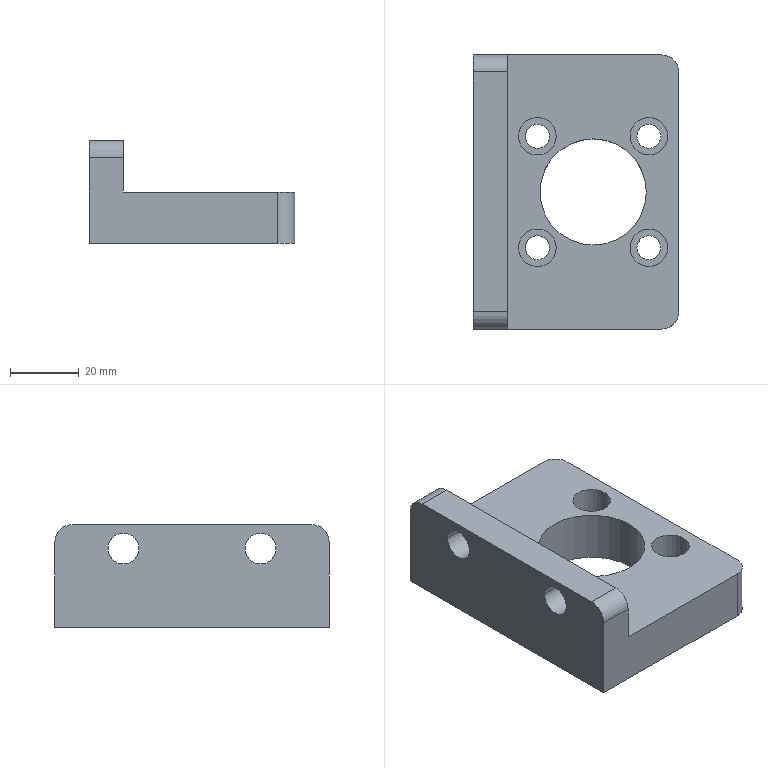Part | 1 solid | 38 faces | box 60 x 80 x 30 mm | volume 67019 mm3 | cylinder 26 | plane 12 | commonest cylinder face diameters 7 x8 11 x8 9 x4 10 x4 31 x2
STEP:
#1=CARTESIAN_POINT('',(-30.,-24.5,23.));
#2=VERTEX_POINT('',#1);
#3=CARTESIAN_POINT('',(-30.,-15.5,23.));
#4=VERTEX_POINT('',#3);
#5=CARTESIAN_POINT('',(-30.,-20.,23.));
#6=DIRECTION('',(1.,0.,0.));
#7=DIRECTION('',(0.,0.,-1.));
#8=AXIS2_PLACEMENT_3D('',#5,#6,#7);
#9=CIRCLE('',#8,4.5);
#10=EDGE_CURVE('',#2,#4,#9,.T.);
#11=ORIENTED_EDGE('',*,*,#10,.F.);
#12=CARTESIAN_POINT('',(-20.,-24.5,23.));
#13=VERTEX_POINT('',#12);
#14=CARTESIAN_POINT('',(-46.,-24.5,23.));
#15=DIRECTION('',(1.,0.,0.));
#16=VECTOR('',#15,1000.);
#17=LINE('',#14,#16);
#18=EDGE_CURVE('',#2,#13,#17,.T.);
#19=ORIENTED_EDGE('',*,*,#18,.T.);
#20=CARTESIAN_POINT('',(-20.,-15.5,23.));
#21=VERTEX_POINT('',#20);
#22=CARTESIAN_POINT('',(-20.,-20.,23.));
#23=DIRECTION('',(1.,0.,0.));
#24=DIRECTION('',(0.,1.,0.));
#25=AXIS2_PLACEMENT_3D('',#22,#23,#24);
#26=CIRCLE('',#25,4.5);
#27=EDGE_CURVE('',#13,#21,#26,.T.);
#28=ORIENTED_EDGE('',*,*,#27,.T.);
#29=CARTESIAN_POINT('',(-46.,-15.5,23.));
#30=DIRECTION('',(1.,0.,0.));
#31=VECTOR('',#30,1000.);
#32=LINE('',#29,#31);
#33=EDGE_CURVE('',#4,#21,#32,.T.);
#34=ORIENTED_EDGE('',*,*,#33,.F.);
#35=EDGE_LOOP('',(#11,#19,#28,#34));
#36=FACE_OUTER_BOUND('',#35,.T.);
#37=CARTESIAN_POINT('',(-46.,-20.,23.));
#38=DIRECTION('',(1.,0.,0.));
#39=DIRECTION('',(0.,1.,0.));
#40=AXIS2_PLACEMENT_3D('',#37,#38,#39);
#41=CYLINDRICAL_SURFACE('',#40,4.5);
#42=ADVANCED_FACE('',(#36),#41,.F.);
#43=CARTESIAN_POINT('',(-30.,15.5,23.));
#44=VERTEX_POINT('',#43);
#45=CARTESIAN_POINT('',(-30.,24.5,23.));
#46=VERTEX_POINT('',#45);
#47=CARTESIAN_POINT('',(-30.,20.,23.));
#48=DIRECTION('',(1.,0.,0.));
#49=DIRECTION('',(0.,0.,-1.));
#50=AXIS2_PLACEMENT_3D('',#47,#48,#49);
#51=CIRCLE('',#50,4.5);
#52=EDGE_CURVE('',#44,#46,#51,.T.);
#53=ORIENTED_EDGE('',*,*,#52,.F.);
#54=CARTESIAN_POINT('',(-20.,15.5,23.));
#55=VERTEX_POINT('',#54);
#56=CARTESIAN_POINT('',(-46.,15.5,23.));
#57=DIRECTION('',(1.,0.,0.));
#58=VECTOR('',#57,1000.);
#59=LINE('',#56,#58);
#60=EDGE_CURVE('',#44,#55,#59,.T.);
#61=ORIENTED_EDGE('',*,*,#60,.T.);
#62=CARTESIAN_POINT('',(-20.,24.5,23.));
#63=VERTEX_POINT('',#62);
#64=CARTESIAN_POINT('',(-20.,20.,23.));
#65=DIRECTION('',(1.,0.,0.));
#66=DIRECTION('',(0.,1.,0.));
#67=AXIS2_PLACEMENT_3D('',#64,#65,#66);
#68=CIRCLE('',#67,4.5);
#69=EDGE_CURVE('',#55,#63,#68,.T.);
#70=ORIENTED_EDGE('',*,*,#69,.T.);
#71=CARTESIAN_POINT('',(-46.,24.5,23.));
#72=DIRECTION('',(1.,0.,0.));
#73=VECTOR('',#72,1000.);
#74=LINE('',#71,#73);
#75=EDGE_CURVE('',#46,#63,#74,.T.);
#76=ORIENTED_EDGE('',*,*,#75,.F.);
#77=EDGE_LOOP('',(#53,#61,#70,#76));
#78=FACE_OUTER_BOUND('',#77,.T.);
#79=CARTESIAN_POINT('',(-46.,20.,23.));
#80=DIRECTION('',(1.,0.,0.));
#81=DIRECTION('',(0.,1.,0.));
#82=AXIS2_PLACEMENT_3D('',#79,#80,#81);
#83=CYLINDRICAL_SURFACE('',#82,4.5);
#84=ADVANCED_FACE('',(#78),#83,.F.);
#85=CARTESIAN_POINT('',(15.763,-16.263,7.));
#86=VERTEX_POINT('',#85);
#87=CARTESIAN_POINT('',(26.763,-16.263,7.));
#88=VERTEX_POINT('',#87);
#89=CARTESIAN_POINT('',(21.263,-16.263,7.));
#90=DIRECTION('',(0.,0.,1.));
#91=DIRECTION('',(1.,0.,0.));
#92=AXIS2_PLACEMENT_3D('',#89,#90,#91);
#93=CIRCLE('',#92,5.5);
#94=EDGE_CURVE('',#86,#88,#93,.T.);
#95=ORIENTED_EDGE('',*,*,#94,.F.);
#96=CARTESIAN_POINT('',(15.763,-16.263,15.));
#97=VERTEX_POINT('',#96);
#98=CARTESIAN_POINT('',(15.763,-16.263,7.));
#99=DIRECTION('',(0.,0.,1.));
#100=VECTOR('',#99,1000.);
#101=LINE('',#98,#100);
#102=EDGE_CURVE('',#86,#97,#101,.T.);
#103=ORIENTED_EDGE('',*,*,#102,.T.);
#104=CARTESIAN_POINT('',(26.763,-16.263,15.));
#105=VERTEX_POINT('',#104);
#106=CARTESIAN_POINT('',(21.263,-16.263,15.));
#107=DIRECTION('',(0.,0.,1.));
#108=DIRECTION('',(1.,0.,0.));
#109=AXIS2_PLACEMENT_3D('',#106,#107,#108);
#110=CIRCLE('',#109,5.5);
#111=EDGE_CURVE('',#97,#105,#110,.T.);
#112=ORIENTED_EDGE('',*,*,#111,.T.);
#113=CARTESIAN_POINT('',(26.763,-16.263,7.));
#114=DIRECTION('',(0.,0.,1.));
#115=VECTOR('',#114,1000.);
#116=LINE('',#113,#115);
#117=EDGE_CURVE('',#88,#105,#116,.T.);
#118=ORIENTED_EDGE('',*,*,#117,.F.);
#119=EDGE_LOOP('',(#95,#103,#112,#118));
#120=FACE_OUTER_BOUND('',#119,.T.);
#121=CARTESIAN_POINT('',(21.263,-16.263,7.));
#122=DIRECTION('',(0.,0.,1.));
#123=DIRECTION('',(1.,0.,0.));
#124=AXIS2_PLACEMENT_3D('',#121,#122,#123);
#125=CYLINDRICAL_SURFACE('',#124,5.5);
#126=ADVANCED_FACE('',(#120),#125,.F.);
#127=CARTESIAN_POINT('',(-16.763,-16.263,7.));
#128=VERTEX_POINT('',#127);
#129=CARTESIAN_POINT('',(-5.763,-16.263,7.));
#130=VERTEX_POINT('',#129);
#131=CARTESIAN_POINT('',(-11.263,-16.263,7.));
#132=DIRECTION('',(0.,0.,1.));
#133=DIRECTION('',(1.,0.,0.));
#134=AXIS2_PLACEMENT_3D('',#131,#132,#133);
#135=CIRCLE('',#134,5.5);
#136=EDGE_CURVE('',#128,#130,#135,.T.);
#137=ORIENTED_EDGE('',*,*,#136,.F.);
#138=CARTESIAN_POINT('',(-16.763,-16.263,15.));
#139=VERTEX_POINT('',#138);
#140=CARTESIAN_POINT('',(-16.763,-16.263,7.));
#141=DIRECTION('',(0.,0.,1.));
#142=VECTOR('',#141,1000.);
#143=LINE('',#140,#142);
#144=EDGE_CURVE('',#128,#139,#143,.T.);
#145=ORIENTED_EDGE('',*,*,#144,.T.);
#146=CARTESIAN_POINT('',(-5.763,-16.263,15.));
#147=VERTEX_POINT('',#146);
#148=CARTESIAN_POINT('',(-11.263,-16.263,15.));
#149=DIRECTION('',(0.,0.,1.));
#150=DIRECTION('',(1.,0.,0.));
#151=AXIS2_PLACEMENT_3D('',#148,#149,#150);
#152=CIRCLE('',#151,5.5);
#153=EDGE_CURVE('',#139,#147,#152,.T.);
#154=ORIENTED_EDGE('',*,*,#153,.T.);
#155=CARTESIAN_POINT('',(-5.763,-16.263,7.));
#156=DIRECTION('',(0.,0.,1.));
#157=VECTOR('',#156,1000.);
#158=LINE('',#155,#157);
#159=EDGE_CURVE('',#130,#147,#158,.T.);
#160=ORIENTED_EDGE('',*,*,#159,.F.);
#161=EDGE_LOOP('',(#137,#145,#154,#160));
#162=FACE_OUTER_BOUND('',#161,.T.);
#163=CARTESIAN_POINT('',(-11.263,-16.263,7.));
#164=DIRECTION('',(0.,0.,1.));
#165=DIRECTION('',(1.,0.,0.));
#166=AXIS2_PLACEMENT_3D('',#163,#164,#165);
#167=CYLINDRICAL_SURFACE('',#166,5.5);
#168=ADVANCED_FACE('',(#162),#167,.F.);
#169=CARTESIAN_POINT('',(15.763,16.263,7.));
#170=VERTEX_POINT('',#169);
#171=CARTESIAN_POINT('',(26.763,16.263,7.));
#172=VERTEX_POINT('',#171);
#173=CARTESIAN_POINT('',(21.263,16.263,7.));
#174=DIRECTION('',(0.,0.,1.));
#175=DIRECTION('',(1.,0.,0.));
#176=AXIS2_PLACEMENT_3D('',#173,#174,#175);
#177=CIRCLE('',#176,5.5);
#178=EDGE_CURVE('',#170,#172,#177,.T.);
#179=ORIENTED_EDGE('',*,*,#178,.F.);
#180=CARTESIAN_POINT('',(15.763,16.263,15.));
#181=VERTEX_POINT('',#180);
#182=CARTESIAN_POINT('',(15.763,16.263,7.));
#183=DIRECTION('',(0.,0.,1.));
#184=VECTOR('',#183,1000.);
#185=LINE('',#182,#184);
#186=EDGE_CURVE('',#170,#181,#185,.T.);
#187=ORIENTED_EDGE('',*,*,#186,.T.);
#188=CARTESIAN_POINT('',(26.763,16.263,15.));
#189=VERTEX_POINT('',#188);
#190=CARTESIAN_POINT('',(21.263,16.263,15.));
#191=DIRECTION('',(0.,0.,1.));
#192=DIRECTION('',(1.,0.,0.));
#193=AXIS2_PLACEMENT_3D('',#190,#191,#192);
#194=CIRCLE('',#193,5.5);
#195=EDGE_CURVE('',#181,#189,#194,.T.);
#196=ORIENTED_EDGE('',*,*,#195,.T.);
#197=CARTESIAN_POINT('',(26.763,16.263,7.));
#198=DIRECTION('',(0.,0.,1.));
#199=VECTOR('',#198,1000.);
#200=LINE('',#197,#199);
#201=EDGE_CURVE('',#172,#189,#200,.T.);
#202=ORIENTED_EDGE('',*,*,#201,.F.);
#203=EDGE_LOOP('',(#179,#187,#196,#202));
#204=FACE_OUTER_BOUND('',#203,.T.);
#205=CARTESIAN_POINT('',(21.263,16.263,7.));
#206=DIRECTION('',(0.,0.,1.));
#207=DIRECTION('',(1.,0.,0.));
#208=AXIS2_PLACEMENT_3D('',#205,#206,#207);
#209=CYLINDRICAL_SURFACE('',#208,5.5);
#210=ADVANCED_FACE('',(#204),#209,.F.);
#211=CARTESIAN_POINT('',(-16.763,16.263,7.));
#212=VERTEX_POINT('',#211);
#213=CARTESIAN_POINT('',(-5.763,16.263,7.));
#214=VERTEX_POINT('',#213);
#215=CARTESIAN_POINT('',(-11.263,16.263,7.));
#216=DIRECTION('',(0.,0.,1.));
#217=DIRECTION('',(1.,0.,0.));
#218=AXIS2_PLACEMENT_3D('',#215,#216,#217);
#219=CIRCLE('',#218,5.5);
#220=EDGE_CURVE('',#212,#214,#219,.T.);
#221=ORIENTED_EDGE('',*,*,#220,.F.);
#222=CARTESIAN_POINT('',(-16.763,16.263,15.));
#223=VERTEX_POINT('',#222);
#224=CARTESIAN_POINT('',(-16.763,16.263,7.));
#225=DIRECTION('',(0.,0.,1.));
#226=VECTOR('',#225,1000.);
#227=LINE('',#224,#226);
#228=EDGE_CURVE('',#212,#223,#227,.T.);
#229=ORIENTED_EDGE('',*,*,#228,.T.);
#230=CARTESIAN_POINT('',(-5.763,16.263,15.));
#231=VERTEX_POINT('',#230);
#232=CARTESIAN_POINT('',(-11.263,16.263,15.));
#233=DIRECTION('',(0.,0.,1.));
#234=DIRECTION('',(1.,0.,0.));
#235=AXIS2_PLACEMENT_3D('',#232,#233,#234);
#236=CIRCLE('',#235,5.5);
#237=EDGE_CURVE('',#223,#231,#236,.T.);
#238=ORIENTED_EDGE('',*,*,#237,.T.);
#239=CARTESIAN_POINT('',(-5.763,16.263,7.));
#240=DIRECTION('',(0.,0.,1.));
#241=VECTOR('',#240,1000.);
#242=LINE('',#239,#241);
#243=EDGE_CURVE('',#214,#231,#242,.T.);
#244=ORIENTED_EDGE('',*,*,#243,.F.);
#245=EDGE_LOOP('',(#221,#229,#238,#244));
#246=FACE_OUTER_BOUND('',#245,.T.);
#247=CARTESIAN_POINT('',(-11.263,16.263,7.));
#248=DIRECTION('',(0.,0.,1.));
#249=DIRECTION('',(1.,0.,0.));
#250=AXIS2_PLACEMENT_3D('',#247,#248,#249);
#251=CYLINDRICAL_SURFACE('',#250,5.5);
#252=ADVANCED_FACE('',(#246),#251,.F.);
#253=CARTESIAN_POINT('',(-10.5,0.,0.));
#254=VERTEX_POINT('',#253);
#255=CARTESIAN_POINT('',(20.5,0.,0.));
#256=VERTEX_POINT('',#255);
#257=CARTESIAN_POINT('',(5.,0.,0.));
#258=DIRECTION('',(0.,0.,1.));
#259=DIRECTION('',(1.,0.,0.));
#260=AXIS2_PLACEMENT_3D('',#257,#258,#259);
#261=CIRCLE('',#260,15.5);
#262=EDGE_CURVE('',#254,#256,#261,.T.);
#263=ORIENTED_EDGE('',*,*,#262,.F.);
#264=CARTESIAN_POINT('',(-10.5,0.,15.));
#265=VERTEX_POINT('',#264);
#266=CARTESIAN_POINT('',(-10.5,0.,0.));
#267=DIRECTION('',(0.,0.,1.));
#268=VECTOR('',#267,1000.);
#269=LINE('',#266,#268);
#270=EDGE_CURVE('',#254,#265,#269,.T.);
#271=ORIENTED_EDGE('',*,*,#270,.T.);
#272=CARTESIAN_POINT('',(20.5,0.,15.));
#273=VERTEX_POINT('',#272);
#274=CARTESIAN_POINT('',(5.,0.,15.));
#275=DIRECTION('',(0.,0.,1.));
#276=DIRECTION('',(1.,0.,0.));
#277=AXIS2_PLACEMENT_3D('',#274,#275,#276);
#278=CIRCLE('',#277,15.5);
#279=EDGE_CURVE('',#265,#273,#278,.T.);
#280=ORIENTED_EDGE('',*,*,#279,.T.);
#281=CARTESIAN_POINT('',(20.5,0.,0.));
#282=DIRECTION('',(0.,0.,1.));
#283=VECTOR('',#282,1000.);
#284=LINE('',#281,#283);
#285=EDGE_CURVE('',#256,#273,#284,.T.);
#286=ORIENTED_EDGE('',*,*,#285,.F.);
#287=EDGE_LOOP('',(#263,#271,#280,#286));
#288=FACE_OUTER_BOUND('',#287,.T.);
#289=CARTESIAN_POINT('',(5.,0.,0.));
#290=DIRECTION('',(0.,0.,1.));
#291=DIRECTION('',(1.,0.,0.));
#292=AXIS2_PLACEMENT_3D('',#289,#290,#291);
#293=CYLINDRICAL_SURFACE('',#292,15.5);
#294=ADVANCED_FACE('',(#288),#293,.F.);
#295=CARTESIAN_POINT('',(-14.763,16.263,0.));
#296=VERTEX_POINT('',#295);
#297=CARTESIAN_POINT('',(-7.763,16.263,0.));
#298=VERTEX_POINT('',#297);
#299=CARTESIAN_POINT('',(-11.263,16.263,0.));
#300=DIRECTION('',(0.,0.,1.));
#301=DIRECTION('',(-1.,0.,0.));
#302=AXIS2_PLACEMENT_3D('',#299,#300,#301);
#303=CIRCLE('',#302,3.5);
#304=EDGE_CURVE('',#296,#298,#303,.T.);
#305=ORIENTED_EDGE('',*,*,#304,.F.);
#306=CARTESIAN_POINT('',(-14.763,16.263,7.));
#307=VERTEX_POINT('',#306);
#308=CARTESIAN_POINT('',(-14.763,16.263,0.));
#309=DIRECTION('',(0.,0.,1.));
#310=VECTOR('',#309,1000.);
#311=LINE('',#308,#310);
#312=EDGE_CURVE('',#296,#307,#311,.T.);
#313=ORIENTED_EDGE('',*,*,#312,.T.);
#314=CARTESIAN_POINT('',(-7.763,16.263,7.));
#315=VERTEX_POINT('',#314);
#316=CARTESIAN_POINT('',(-11.263,16.263,7.));
#317=DIRECTION('',(0.,0.,-1.));
#318=DIRECTION('',(1.,0.,0.));
#319=AXIS2_PLACEMENT_3D('',#316,#317,#318);
#320=CIRCLE('',#319,3.5);
#321=EDGE_CURVE('',#315,#307,#320,.T.);
#322=ORIENTED_EDGE('',*,*,#321,.F.);
#323=CARTESIAN_POINT('',(-7.763,16.263,0.));
#324=DIRECTION('',(0.,0.,1.));
#325=VECTOR('',#324,1000.);
#326=LINE('',#323,#325);
#327=EDGE_CURVE('',#298,#315,#326,.T.);
#328=ORIENTED_EDGE('',*,*,#327,.F.);
#329=EDGE_LOOP('',(#305,#313,#322,#328));
#330=FACE_OUTER_BOUND('',#329,.T.);
#331=CARTESIAN_POINT('',(-11.263,16.263,0.));
#332=DIRECTION('',(0.,0.,1.));
#333=DIRECTION('',(1.,0.,0.));
#334=AXIS2_PLACEMENT_3D('',#331,#332,#333);
#335=CYLINDRICAL_SURFACE('',#334,3.5);
#336=ADVANCED_FACE('',(#330),#335,.F.);
#337=CARTESIAN_POINT('',(17.763,16.263,0.));
#338=VERTEX_POINT('',#337);
#339=CARTESIAN_POINT('',(24.763,16.263,0.));
#340=VERTEX_POINT('',#339);
#341=CARTESIAN_POINT('',(21.263,16.263,0.));
#342=DIRECTION('',(0.,0.,1.));
#343=DIRECTION('',(1.,0.,0.));
#344=AXIS2_PLACEMENT_3D('',#341,#342,#343);
#345=CIRCLE('',#344,3.5);
#346=EDGE_CURVE('',#338,#340,#345,.T.);
#347=ORIENTED_EDGE('',*,*,#346,.F.);
#348=CARTESIAN_POINT('',(17.763,16.263,7.));
#349=VERTEX_POINT('',#348);
#350=CARTESIAN_POINT('',(17.763,16.263,0.));
#351=DIRECTION('',(0.,0.,1.));
#352=VECTOR('',#351,1000.);
#353=LINE('',#350,#352);
#354=EDGE_CURVE('',#338,#349,#353,.T.);
#355=ORIENTED_EDGE('',*,*,#354,.T.);
#356=CARTESIAN_POINT('',(24.763,16.263,7.));
#357=VERTEX_POINT('',#356);
#358=CARTESIAN_POINT('',(21.263,16.263,7.));
#359=DIRECTION('',(0.,0.,-1.));
#360=DIRECTION('',(1.,0.,0.));
#361=AXIS2_PLACEMENT_3D('',#358,#359,#360);
#362=CIRCLE('',#361,3.5);
#363=EDGE_CURVE('',#357,#349,#362,.T.);
#364=ORIENTED_EDGE('',*,*,#363,.F.);
#365=CARTESIAN_POINT('',(24.763,16.263,0.));
#366=DIRECTION('',(0.,0.,1.));
#367=VECTOR('',#366,1000.);
#368=LINE('',#365,#367);
#369=EDGE_CURVE('',#340,#357,#368,.T.);
#370=ORIENTED_EDGE('',*,*,#369,.F.);
#371=EDGE_LOOP('',(#347,#355,#364,#370));
#372=FACE_OUTER_BOUND('',#371,.T.);
#373=CARTESIAN_POINT('',(21.263,16.263,0.));
#374=DIRECTION('',(0.,0.,1.));
#375=DIRECTION('',(1.,0.,0.));
#376=AXIS2_PLACEMENT_3D('',#373,#374,#375);
#377=CYLINDRICAL_SURFACE('',#376,3.5);
#378=ADVANCED_FACE('',(#372),#377,.F.);
#379=CARTESIAN_POINT('',(-14.763,-16.263,0.));
#380=VERTEX_POINT('',#379);
#381=CARTESIAN_POINT('',(-7.763,-16.263,0.));
#382=VERTEX_POINT('',#381);
#383=CARTESIAN_POINT('',(-11.263,-16.263,0.));
#384=DIRECTION('',(0.,0.,1.));
#385=DIRECTION('',(1.,0.,0.));
#386=AXIS2_PLACEMENT_3D('',#383,#384,#385);
#387=CIRCLE('',#386,3.5);
#388=EDGE_CURVE('',#380,#382,#387,.T.);
#389=ORIENTED_EDGE('',*,*,#388,.F.);
#390=CARTESIAN_POINT('',(-14.763,-16.263,7.));
#391=VERTEX_POINT('',#390);
#392=CARTESIAN_POINT('',(-14.763,-16.263,0.));
#393=DIRECTION('',(0.,0.,1.));
#394=VECTOR('',#393,1000.);
#395=LINE('',#392,#394);
#396=EDGE_CURVE('',#380,#391,#395,.T.);
#397=ORIENTED_EDGE('',*,*,#396,.T.);
#398=CARTESIAN_POINT('',(-7.763,-16.263,7.));
#399=VERTEX_POINT('',#398);
#400=CARTESIAN_POINT('',(-11.263,-16.263,7.));
#401=DIRECTION('',(0.,0.,-1.));
#402=DIRECTION('',(1.,0.,0.));
#403=AXIS2_PLACEMENT_3D('',#400,#401,#402);
#404=CIRCLE('',#403,3.5);
#405=EDGE_CURVE('',#399,#391,#404,.T.);
#406=ORIENTED_EDGE('',*,*,#405,.F.);
#407=CARTESIAN_POINT('',(-7.763,-16.263,0.));
#408=DIRECTION('',(0.,0.,1.));
#409=VECTOR('',#408,1000.);
#410=LINE('',#407,#409);
#411=EDGE_CURVE('',#382,#399,#410,.T.);
#412=ORIENTED_EDGE('',*,*,#411,.F.);
#413=EDGE_LOOP('',(#389,#397,#406,#412));
#414=FACE_OUTER_BOUND('',#413,.T.);
#415=CARTESIAN_POINT('',(-11.263,-16.263,0.));
#416=DIRECTION('',(0.,0.,1.));
#417=DIRECTION('',(1.,0.,0.));
#418=AXIS2_PLACEMENT_3D('',#415,#416,#417);
#419=CYLINDRICAL_SURFACE('',#418,3.5);
#420=ADVANCED_FACE('',(#414),#419,.F.);
#421=CARTESIAN_POINT('',(17.763,-16.263,0.));
#422=VERTEX_POINT('',#421);
#423=CARTESIAN_POINT('',(24.763,-16.263,0.));
#424=VERTEX_POINT('',#423);
#425=CARTESIAN_POINT('',(21.263,-16.263,0.));
#426=DIRECTION('',(0.,0.,1.));
#427=DIRECTION('',(-1.,0.,0.));
#428=AXIS2_PLACEMENT_3D('',#425,#426,#427);
#429=CIRCLE('',#428,3.5);
#430=EDGE_CURVE('',#422,#424,#429,.T.);
#431=ORIENTED_EDGE('',*,*,#430,.F.);
#432=CARTESIAN_POINT('',(17.763,-16.263,7.));
#433=VERTEX_POINT('',#432);
#434=CARTESIAN_POINT('',(17.763,-16.263,0.));
#435=DIRECTION('',(0.,0.,1.));
#436=VECTOR('',#435,1000.);
#437=LINE('',#434,#436);
#438=EDGE_CURVE('',#422,#433,#437,.T.);
#439=ORIENTED_EDGE('',*,*,#438,.T.);
#440=CARTESIAN_POINT('',(24.763,-16.263,7.));
#441=VERTEX_POINT('',#440);
#442=CARTESIAN_POINT('',(21.263,-16.263,7.));
#443=DIRECTION('',(0.,0.,-1.));
#444=DIRECTION('',(1.,0.,0.));
#445=AXIS2_PLACEMENT_3D('',#442,#443,#444);
#446=CIRCLE('',#445,3.5);
#447=EDGE_CURVE('',#441,#433,#446,.T.);
#448=ORIENTED_EDGE('',*,*,#447,.F.);
#449=CARTESIAN_POINT('',(24.763,-16.263,0.));
#450=DIRECTION('',(0.,0.,1.));
#451=VECTOR('',#450,1000.);
#452=LINE('',#449,#451);
#453=EDGE_CURVE('',#424,#441,#452,.T.);
#454=ORIENTED_EDGE('',*,*,#453,.F.);
#455=EDGE_LOOP('',(#431,#439,#448,#454));
#456=FACE_OUTER_BOUND('',#455,.T.);
#457=CARTESIAN_POINT('',(21.263,-16.263,0.));
#458=DIRECTION('',(0.,0.,1.));
#459=DIRECTION('',(1.,0.,0.));
#460=AXIS2_PLACEMENT_3D('',#457,#458,#459);
#461=CYLINDRICAL_SURFACE('',#460,3.5);
#462=ADVANCED_FACE('',(#456),#461,.F.);
#463=ORIENTED_EDGE('',*,*,#438,.F.);
#464=CARTESIAN_POINT('',(21.263,-16.263,0.));
#465=DIRECTION('',(0.,0.,1.));
#466=DIRECTION('',(-1.,0.,0.));
#467=AXIS2_PLACEMENT_3D('',#464,#465,#466);
#468=CIRCLE('',#467,3.5);
#469=EDGE_CURVE('',#424,#422,#468,.T.);
#470=ORIENTED_EDGE('',*,*,#469,.F.);
#471=ORIENTED_EDGE('',*,*,#453,.T.);
#472=CARTESIAN_POINT('',(21.263,-16.263,7.));
#473=DIRECTION('',(0.,0.,-1.));
#474=DIRECTION('',(1.,0.,0.));
#475=AXIS2_PLACEMENT_3D('',#472,#473,#474);
#476=CIRCLE('',#475,3.5);
#477=EDGE_CURVE('',#433,#441,#476,.T.);
#478=ORIENTED_EDGE('',*,*,#477,.F.);
#479=EDGE_LOOP('',(#463,#470,#471,#478));
#480=FACE_OUTER_BOUND('',#479,.T.);
#481=CARTESIAN_POINT('',(21.263,-16.263,0.));
#482=DIRECTION('',(0.,0.,1.));
#483=DIRECTION('',(1.,0.,0.));
#484=AXIS2_PLACEMENT_3D('',#481,#482,#483);
#485=CYLINDRICAL_SURFACE('',#484,3.5);
#486=ADVANCED_FACE('',(#480),#485,.F.);
#487=ORIENTED_EDGE('',*,*,#396,.F.);
#488=CARTESIAN_POINT('',(-11.263,-16.263,0.));
#489=DIRECTION('',(0.,0.,1.));
#490=DIRECTION('',(1.,0.,0.));
#491=AXIS2_PLACEMENT_3D('',#488,#489,#490);
#492=CIRCLE('',#491,3.5);
#493=EDGE_CURVE('',#382,#380,#492,.T.);
#494=ORIENTED_EDGE('',*,*,#493,.F.);
#495=ORIENTED_EDGE('',*,*,#411,.T.);
#496=CARTESIAN_POINT('',(-11.263,-16.263,7.));
#497=DIRECTION('',(0.,0.,-1.));
#498=DIRECTION('',(1.,0.,0.));
#499=AXIS2_PLACEMENT_3D('',#496,#497,#498);
#500=CIRCLE('',#499,3.5);
#501=EDGE_CURVE('',#391,#399,#500,.T.);
#502=ORIENTED_EDGE('',*,*,#501,.F.);
#503=EDGE_LOOP('',(#487,#494,#495,#502));
#504=FACE_OUTER_BOUND('',#503,.T.);
#505=CARTESIAN_POINT('',(-11.263,-16.263,0.));
#506=DIRECTION('',(0.,0.,1.));
#507=DIRECTION('',(1.,0.,0.));
#508=AXIS2_PLACEMENT_3D('',#505,#506,#507);
#509=CYLINDRICAL_SURFACE('',#508,3.5);
#510=ADVANCED_FACE('',(#504),#509,.F.);
#511=ORIENTED_EDGE('',*,*,#354,.F.);
#512=CARTESIAN_POINT('',(21.263,16.263,0.));
#513=DIRECTION('',(0.,0.,1.));
#514=DIRECTION('',(1.,0.,0.));
#515=AXIS2_PLACEMENT_3D('',#512,#513,#514);
#516=CIRCLE('',#515,3.5);
#517=EDGE_CURVE('',#340,#338,#516,.T.);
#518=ORIENTED_EDGE('',*,*,#517,.F.);
#519=ORIENTED_EDGE('',*,*,#369,.T.);
#520=CARTESIAN_POINT('',(21.263,16.263,7.));
#521=DIRECTION('',(0.,0.,-1.));
#522=DIRECTION('',(1.,0.,0.));
#523=AXIS2_PLACEMENT_3D('',#520,#521,#522);
#524=CIRCLE('',#523,3.5);
#525=EDGE_CURVE('',#349,#357,#524,.T.);
#526=ORIENTED_EDGE('',*,*,#525,.F.);
#527=EDGE_LOOP('',(#511,#518,#519,#526));
#528=FACE_OUTER_BOUND('',#527,.T.);
#529=CARTESIAN_POINT('',(21.263,16.263,0.));
#530=DIRECTION('',(0.,0.,1.));
#531=DIRECTION('',(1.,0.,0.));
#532=AXIS2_PLACEMENT_3D('',#529,#530,#531);
#533=CYLINDRICAL_SURFACE('',#532,3.5);
#534=ADVANCED_FACE('',(#528),#533,.F.);
#535=ORIENTED_EDGE('',*,*,#312,.F.);
#536=CARTESIAN_POINT('',(-11.263,16.263,0.));
#537=DIRECTION('',(0.,0.,1.));
#538=DIRECTION('',(-1.,0.,0.));
#539=AXIS2_PLACEMENT_3D('',#536,#537,#538);
#540=CIRCLE('',#539,3.5);
#541=EDGE_CURVE('',#298,#296,#540,.T.);
#542=ORIENTED_EDGE('',*,*,#541,.F.);
#543=ORIENTED_EDGE('',*,*,#327,.T.);
#544=CARTESIAN_POINT('',(-11.263,16.263,7.));
#545=DIRECTION('',(0.,0.,-1.));
#546=DIRECTION('',(1.,0.,0.));
#547=AXIS2_PLACEMENT_3D('',#544,#545,#546);
#548=CIRCLE('',#547,3.5);
#549=EDGE_CURVE('',#307,#315,#548,.T.);
#550=ORIENTED_EDGE('',*,*,#549,.F.);
#551=EDGE_LOOP('',(#535,#542,#543,#550));
#552=FACE_OUTER_BOUND('',#551,.T.);
#553=CARTESIAN_POINT('',(-11.263,16.263,0.));
#554=DIRECTION('',(0.,0.,1.));
#555=DIRECTION('',(1.,0.,0.));
#556=AXIS2_PLACEMENT_3D('',#553,#554,#555);
#557=CYLINDRICAL_SURFACE('',#556,3.5);
#558=ADVANCED_FACE('',(#552),#557,.F.);
#559=CARTESIAN_POINT('',(21.263,-16.263,15.));
#560=DIRECTION('',(0.,0.,1.));
#561=DIRECTION('',(1.,0.,0.));
#562=AXIS2_PLACEMENT_3D('',#559,#560,#561);
#563=CIRCLE('',#562,5.5);
#564=EDGE_CURVE('',#105,#97,#563,.T.);
#565=ORIENTED_EDGE('',*,*,#564,.F.);
#566=ORIENTED_EDGE('',*,*,#111,.F.);
#567=EDGE_LOOP('',(#565,#566));
#568=FACE_BOUND('',#567,.T.);
#569=CARTESIAN_POINT('',(-11.263,-16.263,15.));
#570=DIRECTION('',(0.,0.,1.));
#571=DIRECTION('',(1.,0.,0.));
#572=AXIS2_PLACEMENT_3D('',#569,#570,#571);
#573=CIRCLE('',#572,5.5);
#574=EDGE_CURVE('',#147,#139,#573,.T.);
#575=ORIENTED_EDGE('',*,*,#574,.F.);
#576=ORIENTED_EDGE('',*,*,#153,.F.);
#577=EDGE_LOOP('',(#575,#576));
#578=FACE_BOUND('',#577,.T.);
#579=CARTESIAN_POINT('',(21.263,16.263,15.));
#580=DIRECTION('',(0.,0.,1.));
#581=DIRECTION('',(1.,0.,0.));
#582=AXIS2_PLACEMENT_3D('',#579,#580,#581);
#583=CIRCLE('',#582,5.5);
#584=EDGE_CURVE('',#189,#181,#583,.T.);
#585=ORIENTED_EDGE('',*,*,#584,.F.);
#586=ORIENTED_EDGE('',*,*,#195,.F.);
#587=EDGE_LOOP('',(#585,#586));
#588=FACE_BOUND('',#587,.T.);
#589=CARTESIAN_POINT('',(-11.263,16.263,15.));
#590=DIRECTION('',(0.,0.,1.));
#591=DIRECTION('',(1.,0.,0.));
#592=AXIS2_PLACEMENT_3D('',#589,#590,#591);
#593=CIRCLE('',#592,5.5);
#594=EDGE_CURVE('',#231,#223,#593,.T.);
#595=ORIENTED_EDGE('',*,*,#594,.F.);
#596=ORIENTED_EDGE('',*,*,#237,.F.);
#597=EDGE_LOOP('',(#595,#596));
#598=FACE_BOUND('',#597,.T.);
#599=CARTESIAN_POINT('',(5.,0.,15.));
#600=DIRECTION('',(0.,0.,1.));
#601=DIRECTION('',(1.,0.,0.));
#602=AXIS2_PLACEMENT_3D('',#599,#600,#601);
#603=CIRCLE('',#602,15.5);
#604=EDGE_CURVE('',#273,#265,#603,.T.);
#605=ORIENTED_EDGE('',*,*,#604,.F.);
#606=ORIENTED_EDGE('',*,*,#279,.F.);
#607=EDGE_LOOP('',(#605,#606));
#608=FACE_BOUND('',#607,.T.);
#609=CARTESIAN_POINT('',(-20.,-40.,15.));
#610=VERTEX_POINT('',#609);
#611=CARTESIAN_POINT('',(25.,-40.,15.));
#612=VERTEX_POINT('',#611);
#613=CARTESIAN_POINT('',(-30.,-40.,15.));
#614=DIRECTION('',(1.,0.,0.));
#615=VECTOR('',#614,1000.);
#616=LINE('',#613,#615);
#617=EDGE_CURVE('',#610,#612,#616,.T.);
#618=ORIENTED_EDGE('',*,*,#617,.T.);
#619=CARTESIAN_POINT('',(30.,-35.,15.));
#620=VERTEX_POINT('',#619);
#621=CARTESIAN_POINT('',(25.,-35.,15.));
#622=DIRECTION('',(0.,0.,1.));
#623=DIRECTION('',(-1.,0.,0.));
#624=AXIS2_PLACEMENT_3D('',#621,#622,#623);
#625=CIRCLE('',#624,5.);
#626=EDGE_CURVE('',#612,#620,#625,.T.);
#627=ORIENTED_EDGE('',*,*,#626,.T.);
#628=CARTESIAN_POINT('',(30.,35.,15.));
#629=VERTEX_POINT('',#628);
#630=CARTESIAN_POINT('',(30.,-40.,15.));
#631=DIRECTION('',(0.,1.,0.));
#632=VECTOR('',#631,1000.);
#633=LINE('',#630,#632);
#634=EDGE_CURVE('',#620,#629,#633,.T.);
#635=ORIENTED_EDGE('',*,*,#634,.T.);
#636=CARTESIAN_POINT('',(25.,40.,15.));
#637=VERTEX_POINT('',#636);
#638=CARTESIAN_POINT('',(25.,35.,15.));
#639=DIRECTION('',(0.,0.,1.));
#640=DIRECTION('',(-1.,0.,0.));
#641=AXIS2_PLACEMENT_3D('',#638,#639,#640);
#642=CIRCLE('',#641,5.);
#643=EDGE_CURVE('',#629,#637,#642,.T.);
#644=ORIENTED_EDGE('',*,*,#643,.T.);
#645=CARTESIAN_POINT('',(-20.,40.,15.));
#646=VERTEX_POINT('',#645);
#647=CARTESIAN_POINT('',(-30.,40.,15.));
#648=DIRECTION('',(-1.,0.,0.));
#649=VECTOR('',#648,1000.);
#650=LINE('',#647,#649);
#651=EDGE_CURVE('',#637,#646,#650,.T.);
#652=ORIENTED_EDGE('',*,*,#651,.T.);
#653=CARTESIAN_POINT('',(-20.,-40.,15.));
#654=DIRECTION('',(0.,1.,0.));
#655=VECTOR('',#654,1000.);
#656=LINE('',#653,#655);
#657=EDGE_CURVE('',#610,#646,#656,.T.);
#658=ORIENTED_EDGE('',*,*,#657,.F.);
#659=EDGE_LOOP('',(#618,#627,#635,#644,#652,#658));
#660=FACE_OUTER_BOUND('',#659,.T.);
#661=CARTESIAN_POINT('',(0.,0.,15.));
#662=DIRECTION('',(0.,0.,-1.));
#663=DIRECTION('',(-1.,0.,0.));
#664=AXIS2_PLACEMENT_3D('',#661,#662,#663);
#665=PLANE('',#664);
#666=ADVANCED_FACE('',(#568,#578,#588,#598,#608,#660),#665,.F.);
#667=ORIENTED_EDGE('',*,*,#634,.F.);
#668=CARTESIAN_POINT('',(30.,-35.,0.));
#669=VERTEX_POINT('',#668);
#670=CARTESIAN_POINT('',(30.,-35.,15.));
#671=DIRECTION('',(0.,0.,-1.));
#672=VECTOR('',#671,1000.);
#673=LINE('',#670,#672);
#674=EDGE_CURVE('',#620,#669,#673,.T.);
#675=ORIENTED_EDGE('',*,*,#674,.T.);
#676=CARTESIAN_POINT('',(30.,35.,0.));
#677=VERTEX_POINT('',#676);
#678=CARTESIAN_POINT('',(30.,-40.,0.));
#679=DIRECTION('',(0.,1.,0.));
#680=VECTOR('',#679,1000.);
#681=LINE('',#678,#680);
#682=EDGE_CURVE('',#669,#677,#681,.T.);
#683=ORIENTED_EDGE('',*,*,#682,.T.);
#684=CARTESIAN_POINT('',(30.,35.,15.));
#685=DIRECTION('',(0.,0.,1.));
#686=VECTOR('',#685,1000.);
#687=LINE('',#684,#686);
#688=EDGE_CURVE('',#677,#629,#687,.T.);
#689=ORIENTED_EDGE('',*,*,#688,.T.);
#690=EDGE_LOOP('',(#667,#675,#683,#689));
#691=FACE_OUTER_BOUND('',#690,.T.);
#692=CARTESIAN_POINT('',(30.,-40.,15.));
#693=DIRECTION('',(-1.,0.,0.));
#694=DIRECTION('',(0.,0.,1.));
#695=AXIS2_PLACEMENT_3D('',#692,#693,#694);
#696=PLANE('',#695);
#697=ADVANCED_FACE('',(#691),#696,.F.);
#698=ORIENTED_EDGE('',*,*,#651,.F.);
#699=CARTESIAN_POINT('',(25.,40.,0.));
#700=VERTEX_POINT('',#699);
#701=CARTESIAN_POINT('',(25.,40.,15.));
#702=DIRECTION('',(0.,0.,-1.));
#703=VECTOR('',#702,1000.);
#704=LINE('',#701,#703);
#705=EDGE_CURVE('',#637,#700,#704,.T.);
#706=ORIENTED_EDGE('',*,*,#705,.T.);
#707=CARTESIAN_POINT('',(-30.,40.,0.));
#708=VERTEX_POINT('',#707);
#709=CARTESIAN_POINT('',(-30.,40.,0.));
#710=DIRECTION('',(-1.,0.,0.));
#711=VECTOR('',#710,1000.);
#712=LINE('',#709,#711);
#713=EDGE_CURVE('',#700,#708,#712,.T.);
#714=ORIENTED_EDGE('',*,*,#713,.T.);
#715=CARTESIAN_POINT('',(-30.,40.,25.));
#716=VERTEX_POINT('',#715);
#717=CARTESIAN_POINT('',(-30.,40.,15.));
#718=DIRECTION('',(0.,0.,-1.));
#719=VECTOR('',#718,1000.);
#720=LINE('',#717,#719);
#721=EDGE_CURVE('',#716,#708,#720,.T.);
#722=ORIENTED_EDGE('',*,*,#721,.F.);
#723=CARTESIAN_POINT('',(-20.,40.,25.));
#724=VERTEX_POINT('',#723);
#725=CARTESIAN_POINT('',(-30.,40.,25.));
#726=DIRECTION('',(1.,0.,0.));
#727=VECTOR('',#726,1000.);
#728=LINE('',#725,#727);
#729=EDGE_CURVE('',#716,#724,#728,.T.);
#730=ORIENTED_EDGE('',*,*,#729,.T.);
#731=CARTESIAN_POINT('',(-20.,40.,30.));
#732=DIRECTION('',(0.,0.,-1.));
#733=VECTOR('',#732,1000.);
#734=LINE('',#731,#733);
#735=EDGE_CURVE('',#724,#646,#734,.T.);
#736=ORIENTED_EDGE('',*,*,#735,.T.);
#737=EDGE_LOOP('',(#698,#706,#714,#722,#730,#736));
#738=FACE_OUTER_BOUND('',#737,.T.);
#739=CARTESIAN_POINT('',(-30.,40.,15.));
#740=DIRECTION('',(0.,-1.,0.));
#741=DIRECTION('',(0.,0.,-1.));
#742=AXIS2_PLACEMENT_3D('',#739,#740,#741);
#743=PLANE('',#742);
#744=ADVANCED_FACE('',(#738),#743,.F.);
#745=CARTESIAN_POINT('',(-30.,-20.,23.));
#746=DIRECTION('',(1.,0.,0.));
#747=DIRECTION('',(0.,0.,-1.));
#748=AXIS2_PLACEMENT_3D('',#745,#746,#747);
#749=CIRCLE('',#748,4.5);
#750=EDGE_CURVE('',#4,#2,#749,.T.);
#751=ORIENTED_EDGE('',*,*,#750,.T.);
#752=ORIENTED_EDGE('',*,*,#10,.T.);
#753=EDGE_LOOP('',(#751,#752));
#754=FACE_BOUND('',#753,.T.);
#755=CARTESIAN_POINT('',(-30.,20.,23.));
#756=DIRECTION('',(1.,0.,0.));
#757=DIRECTION('',(0.,0.,-1.));
#758=AXIS2_PLACEMENT_3D('',#755,#756,#757);
#759=CIRCLE('',#758,4.5);
#760=EDGE_CURVE('',#46,#44,#759,.T.);
#761=ORIENTED_EDGE('',*,*,#760,.T.);
#762=ORIENTED_EDGE('',*,*,#52,.T.);
#763=EDGE_LOOP('',(#761,#762));
#764=FACE_BOUND('',#763,.T.);
#765=CARTESIAN_POINT('',(-30.,35.,30.));
#766=VERTEX_POINT('',#765);
#767=CARTESIAN_POINT('',(-30.,-35.,30.));
#768=VERTEX_POINT('',#767);
#769=CARTESIAN_POINT('',(-30.,-40.,30.));
#770=DIRECTION('',(0.,-1.,0.));
#771=VECTOR('',#770,1000.);
#772=LINE('',#769,#771);
#773=EDGE_CURVE('',#766,#768,#772,.T.);
#774=ORIENTED_EDGE('',*,*,#773,.F.);
#775=CARTESIAN_POINT('',(-30.,35.,25.));
#776=DIRECTION('',(-1.,0.,0.));
#777=DIRECTION('',(0.,0.,-1.));
#778=AXIS2_PLACEMENT_3D('',#775,#776,#777);
#779=CIRCLE('',#778,5.);
#780=EDGE_CURVE('',#766,#716,#779,.T.);
#781=ORIENTED_EDGE('',*,*,#780,.T.);
#782=ORIENTED_EDGE('',*,*,#721,.T.);
#783=CARTESIAN_POINT('',(-30.,-40.,0.));
#784=VERTEX_POINT('',#783);
#785=CARTESIAN_POINT('',(-30.,-40.,0.));
#786=DIRECTION('',(0.,-1.,0.));
#787=VECTOR('',#786,1000.);
#788=LINE('',#785,#787);
#789=EDGE_CURVE('',#708,#784,#788,.T.);
#790=ORIENTED_EDGE('',*,*,#789,.T.);
#791=CARTESIAN_POINT('',(-30.,-40.,25.));
#792=VERTEX_POINT('',#791);
#793=CARTESIAN_POINT('',(-30.,-40.,15.));
#794=DIRECTION('',(0.,0.,-1.));
#795=VECTOR('',#794,1000.);
#796=LINE('',#793,#795);
#797=EDGE_CURVE('',#792,#784,#796,.T.);
#798=ORIENTED_EDGE('',*,*,#797,.F.);
#799=CARTESIAN_POINT('',(-30.,-35.,25.));
#800=DIRECTION('',(-1.,0.,0.));
#801=DIRECTION('',(0.,0.,-1.));
#802=AXIS2_PLACEMENT_3D('',#799,#800,#801);
#803=CIRCLE('',#802,5.);
#804=EDGE_CURVE('',#792,#768,#803,.T.);
#805=ORIENTED_EDGE('',*,*,#804,.T.);
#806=EDGE_LOOP('',(#774,#781,#782,#790,#798,#805));
#807=FACE_OUTER_BOUND('',#806,.T.);
#808=CARTESIAN_POINT('',(-30.,-40.,15.));
#809=DIRECTION('',(1.,0.,0.));
#810=DIRECTION('',(0.,0.,-1.));
#811=AXIS2_PLACEMENT_3D('',#808,#809,#810);
#812=PLANE('',#811);
#813=ADVANCED_FACE('',(#754,#764,#807),#812,.F.);
#814=CARTESIAN_POINT('',(25.,-40.,0.));
#815=VERTEX_POINT('',#814);
#816=CARTESIAN_POINT('',(-30.,-40.,0.));
#817=DIRECTION('',(1.,0.,0.));
#818=VECTOR('',#817,1000.);
#819=LINE('',#816,#818);
#820=EDGE_CURVE('',#784,#815,#819,.T.);
#821=ORIENTED_EDGE('',*,*,#820,.T.);
#822=CARTESIAN_POINT('',(25.,-40.,15.));
#823=DIRECTION('',(0.,0.,1.));
#824=VECTOR('',#823,1000.);
#825=LINE('',#822,#824);
#826=EDGE_CURVE('',#815,#612,#825,.T.);
#827=ORIENTED_EDGE('',*,*,#826,.T.);
#828=ORIENTED_EDGE('',*,*,#617,.F.);
#829=CARTESIAN_POINT('',(-20.,-40.,25.));
#830=VERTEX_POINT('',#829);
#831=CARTESIAN_POINT('',(-20.,-40.,30.));
#832=DIRECTION('',(0.,0.,-1.));
#833=VECTOR('',#832,1000.);
#834=LINE('',#831,#833);
#835=EDGE_CURVE('',#830,#610,#834,.T.);
#836=ORIENTED_EDGE('',*,*,#835,.F.);
#837=CARTESIAN_POINT('',(-30.,-40.,25.));
#838=DIRECTION('',(-1.,0.,0.));
#839=VECTOR('',#838,1000.);
#840=LINE('',#837,#839);
#841=EDGE_CURVE('',#830,#792,#840,.T.);
#842=ORIENTED_EDGE('',*,*,#841,.T.);
#843=ORIENTED_EDGE('',*,*,#797,.T.);
#844=EDGE_LOOP('',(#821,#827,#828,#836,#842,#843));
#845=FACE_OUTER_BOUND('',#844,.T.);
#846=CARTESIAN_POINT('',(-30.,-40.,15.));
#847=DIRECTION('',(0.,1.,0.));
#848=DIRECTION('',(0.,0.,1.));
#849=AXIS2_PLACEMENT_3D('',#846,#847,#848);
#850=PLANE('',#849);
#851=ADVANCED_FACE('',(#845),#850,.F.);
#852=ORIENTED_EDGE('',*,*,#469,.T.);
#853=ORIENTED_EDGE('',*,*,#430,.T.);
#854=EDGE_LOOP('',(#852,#853));
#855=FACE_BOUND('',#854,.T.);
#856=ORIENTED_EDGE('',*,*,#493,.T.);
#857=ORIENTED_EDGE('',*,*,#388,.T.);
#858=EDGE_LOOP('',(#856,#857));
#859=FACE_BOUND('',#858,.T.);
#860=ORIENTED_EDGE('',*,*,#541,.T.);
#861=ORIENTED_EDGE('',*,*,#304,.T.);
#862=EDGE_LOOP('',(#860,#861));
#863=FACE_BOUND('',#862,.T.);
#864=ORIENTED_EDGE('',*,*,#517,.T.);
#865=ORIENTED_EDGE('',*,*,#346,.T.);
#866=EDGE_LOOP('',(#864,#865));
#867=FACE_BOUND('',#866,.T.);
#868=CARTESIAN_POINT('',(5.,0.,0.));
#869=DIRECTION('',(0.,0.,1.));
#870=DIRECTION('',(1.,0.,0.));
#871=AXIS2_PLACEMENT_3D('',#868,#869,#870);
#872=CIRCLE('',#871,15.5);
#873=EDGE_CURVE('',#256,#254,#872,.T.);
#874=ORIENTED_EDGE('',*,*,#873,.T.);
#875=ORIENTED_EDGE('',*,*,#262,.T.);
#876=EDGE_LOOP('',(#874,#875));
#877=FACE_BOUND('',#876,.T.);
#878=ORIENTED_EDGE('',*,*,#682,.F.);
#879=CARTESIAN_POINT('',(25.,-35.,0.));
#880=DIRECTION('',(0.,0.,-1.));
#881=DIRECTION('',(-1.,0.,0.));
#882=AXIS2_PLACEMENT_3D('',#879,#880,#881);
#883=CIRCLE('',#882,5.);
#884=EDGE_CURVE('',#669,#815,#883,.T.);
#885=ORIENTED_EDGE('',*,*,#884,.T.);
#886=ORIENTED_EDGE('',*,*,#820,.F.);
#887=ORIENTED_EDGE('',*,*,#789,.F.);
#888=ORIENTED_EDGE('',*,*,#713,.F.);
#889=CARTESIAN_POINT('',(25.,35.,0.));
#890=DIRECTION('',(0.,0.,-1.));
#891=DIRECTION('',(-1.,0.,0.));
#892=AXIS2_PLACEMENT_3D('',#889,#890,#891);
#893=CIRCLE('',#892,5.);
#894=EDGE_CURVE('',#700,#677,#893,.T.);
#895=ORIENTED_EDGE('',*,*,#894,.T.);
#896=EDGE_LOOP('',(#878,#885,#886,#887,#888,#895));
#897=FACE_OUTER_BOUND('',#896,.T.);
#898=CARTESIAN_POINT('',(0.,0.,0.));
#899=DIRECTION('',(0.,0.,-1.));
#900=DIRECTION('',(-1.,0.,0.));
#901=AXIS2_PLACEMENT_3D('',#898,#899,#900);
#902=PLANE('',#901);
#903=ADVANCED_FACE('',(#855,#859,#863,#867,#877,#897),#902,.T.);
#904=CARTESIAN_POINT('',(-20.,-20.,23.));
#905=DIRECTION('',(1.,0.,0.));
#906=DIRECTION('',(0.,1.,0.));
#907=AXIS2_PLACEMENT_3D('',#904,#905,#906);
#908=CIRCLE('',#907,4.5);
#909=EDGE_CURVE('',#21,#13,#908,.T.);
#910=ORIENTED_EDGE('',*,*,#909,.F.);
#911=ORIENTED_EDGE('',*,*,#27,.F.);
#912=EDGE_LOOP('',(#910,#911));
#913=FACE_BOUND('',#912,.T.);
#914=CARTESIAN_POINT('',(-20.,20.,23.));
#915=DIRECTION('',(1.,0.,0.));
#916=DIRECTION('',(0.,1.,0.));
#917=AXIS2_PLACEMENT_3D('',#914,#915,#916);
#918=CIRCLE('',#917,4.5);
#919=EDGE_CURVE('',#63,#55,#918,.T.);
#920=ORIENTED_EDGE('',*,*,#919,.F.);
#921=ORIENTED_EDGE('',*,*,#69,.F.);
#922=EDGE_LOOP('',(#920,#921));
#923=FACE_BOUND('',#922,.T.);
#924=ORIENTED_EDGE('',*,*,#735,.F.);
#925=CARTESIAN_POINT('',(-20.,35.,30.));
#926=VERTEX_POINT('',#925);
#927=CARTESIAN_POINT('',(-20.,35.,25.));
#928=DIRECTION('',(1.,0.,0.));
#929=DIRECTION('',(0.,-1.,0.));
#930=AXIS2_PLACEMENT_3D('',#927,#928,#929);
#931=CIRCLE('',#930,5.);
#932=EDGE_CURVE('',#724,#926,#931,.T.);
#933=ORIENTED_EDGE('',*,*,#932,.T.);
#934=CARTESIAN_POINT('',(-20.,-35.,30.));
#935=VERTEX_POINT('',#934);
#936=CARTESIAN_POINT('',(-20.,-40.,30.));
#937=DIRECTION('',(0.,1.,0.));
#938=VECTOR('',#937,1000.);
#939=LINE('',#936,#938);
#940=EDGE_CURVE('',#935,#926,#939,.T.);
#941=ORIENTED_EDGE('',*,*,#940,.F.);
#942=CARTESIAN_POINT('',(-20.,-35.,25.));
#943=DIRECTION('',(1.,0.,0.));
#944=DIRECTION('',(0.,-1.,0.));
#945=AXIS2_PLACEMENT_3D('',#942,#943,#944);
#946=CIRCLE('',#945,5.);
#947=EDGE_CURVE('',#935,#830,#946,.T.);
#948=ORIENTED_EDGE('',*,*,#947,.T.);
#949=ORIENTED_EDGE('',*,*,#835,.T.);
#950=ORIENTED_EDGE('',*,*,#657,.T.);
#951=EDGE_LOOP('',(#924,#933,#941,#948,#949,#950));
#952=FACE_OUTER_BOUND('',#951,.T.);
#953=CARTESIAN_POINT('',(-20.,-40.,30.));
#954=DIRECTION('',(-1.,0.,0.));
#955=DIRECTION('',(0.,-1.,0.));
#956=AXIS2_PLACEMENT_3D('',#953,#954,#955);
#957=PLANE('',#956);
#958=ADVANCED_FACE('',(#913,#923,#952),#957,.F.);
#959=ORIENTED_EDGE('',*,*,#940,.T.);
#960=CARTESIAN_POINT('',(0.,35.,30.));
#961=DIRECTION('',(-1.,0.,0.));
#962=VECTOR('',#961,1000.);
#963=LINE('',#960,#962);
#964=EDGE_CURVE('',#926,#766,#963,.T.);
#965=ORIENTED_EDGE('',*,*,#964,.T.);
#966=ORIENTED_EDGE('',*,*,#773,.T.);
#967=CARTESIAN_POINT('',(0.,-35.,30.));
#968=DIRECTION('',(1.,0.,0.));
#969=VECTOR('',#968,1000.);
#970=LINE('',#967,#969);
#971=EDGE_CURVE('',#768,#935,#970,.T.);
#972=ORIENTED_EDGE('',*,*,#971,.T.);
#973=EDGE_LOOP('',(#959,#965,#966,#972));
#974=FACE_OUTER_BOUND('',#973,.T.);
#975=CARTESIAN_POINT('',(0.,0.,30.));
#976=DIRECTION('',(0.,0.,-1.));
#977=DIRECTION('',(-1.,0.,0.));
#978=AXIS2_PLACEMENT_3D('',#975,#976,#977);
#979=PLANE('',#978);
#980=ADVANCED_FACE('',(#974),#979,.F.);
#981=ORIENTED_EDGE('',*,*,#270,.F.);
#982=ORIENTED_EDGE('',*,*,#873,.F.);
#983=ORIENTED_EDGE('',*,*,#285,.T.);
#984=ORIENTED_EDGE('',*,*,#604,.T.);
#985=EDGE_LOOP('',(#981,#982,#983,#984));
#986=FACE_OUTER_BOUND('',#985,.T.);
#987=CARTESIAN_POINT('',(5.,0.,0.));
#988=DIRECTION('',(0.,0.,1.));
#989=DIRECTION('',(1.,0.,0.));
#990=AXIS2_PLACEMENT_3D('',#987,#988,#989);
#991=CYLINDRICAL_SURFACE('',#990,15.5);
#992=ADVANCED_FACE('',(#986),#991,.F.);
#993=CARTESIAN_POINT('',(-11.263,16.263,7.));
#994=DIRECTION('',(0.,0.,1.));
#995=DIRECTION('',(1.,0.,0.));
#996=AXIS2_PLACEMENT_3D('',#993,#994,#995);
#997=CIRCLE('',#996,5.5);
#998=EDGE_CURVE('',#214,#212,#997,.T.);
#999=ORIENTED_EDGE('',*,*,#998,.T.);
#1000=ORIENTED_EDGE('',*,*,#220,.T.);
#1001=EDGE_LOOP('',(#999,#1000));
#1002=FACE_OUTER_BOUND('',#1001,.T.);
#1003=ORIENTED_EDGE('',*,*,#321,.T.);
#1004=ORIENTED_EDGE('',*,*,#549,.T.);
#1005=EDGE_LOOP('',(#1003,#1004));
#1006=FACE_BOUND('',#1005,.T.);
#1007=CARTESIAN_POINT('',(-11.263,16.263,7.));
#1008=DIRECTION('',(0.,0.,1.));
#1009=DIRECTION('',(1.,0.,0.));
#1010=AXIS2_PLACEMENT_3D('',#1007,#1008,#1009);
#1011=PLANE('',#1010);
#1012=ADVANCED_FACE('',(#1002,#1006),#1011,.T.);
#1013=ORIENTED_EDGE('',*,*,#228,.F.);
#1014=ORIENTED_EDGE('',*,*,#998,.F.);
#1015=ORIENTED_EDGE('',*,*,#243,.T.);
#1016=ORIENTED_EDGE('',*,*,#594,.T.);
#1017=EDGE_LOOP('',(#1013,#1014,#1015,#1016));
#1018=FACE_OUTER_BOUND('',#1017,.T.);
#1019=CARTESIAN_POINT('',(-11.263,16.263,7.));
#1020=DIRECTION('',(0.,0.,1.));
#1021=DIRECTION('',(1.,0.,0.));
#1022=AXIS2_PLACEMENT_3D('',#1019,#1020,#1021);
#1023=CYLINDRICAL_SURFACE('',#1022,5.5);
#1024=ADVANCED_FACE('',(#1018),#1023,.F.);
#1025=CARTESIAN_POINT('',(21.263,16.263,7.));
#1026=DIRECTION('',(0.,0.,1.));
#1027=DIRECTION('',(1.,0.,0.));
#1028=AXIS2_PLACEMENT_3D('',#1025,#1026,#1027);
#1029=CIRCLE('',#1028,5.5);
#1030=EDGE_CURVE('',#172,#170,#1029,.T.);
#1031=ORIENTED_EDGE('',*,*,#1030,.T.);
#1032=ORIENTED_EDGE('',*,*,#178,.T.);
#1033=EDGE_LOOP('',(#1031,#1032));
#1034=FACE_OUTER_BOUND('',#1033,.T.);
#1035=ORIENTED_EDGE('',*,*,#363,.T.);
#1036=ORIENTED_EDGE('',*,*,#525,.T.);
#1037=EDGE_LOOP('',(#1035,#1036));
#1038=FACE_BOUND('',#1037,.T.);
#1039=CARTESIAN_POINT('',(21.263,16.263,7.));
#1040=DIRECTION('',(0.,0.,1.));
#1041=DIRECTION('',(1.,0.,0.));
#1042=AXIS2_PLACEMENT_3D('',#1039,#1040,#1041);
#1043=PLANE('',#1042);
#1044=ADVANCED_FACE('',(#1034,#1038),#1043,.T.);
#1045=ORIENTED_EDGE('',*,*,#186,.F.);
#1046=ORIENTED_EDGE('',*,*,#1030,.F.);
#1047=ORIENTED_EDGE('',*,*,#201,.T.);
#1048=ORIENTED_EDGE('',*,*,#584,.T.);
#1049=EDGE_LOOP('',(#1045,#1046,#1047,#1048));
#1050=FACE_OUTER_BOUND('',#1049,.T.);
#1051=CARTESIAN_POINT('',(21.263,16.263,7.));
#1052=DIRECTION('',(0.,0.,1.));
#1053=DIRECTION('',(1.,0.,0.));
#1054=AXIS2_PLACEMENT_3D('',#1051,#1052,#1053);
#1055=CYLINDRICAL_SURFACE('',#1054,5.5);
#1056=ADVANCED_FACE('',(#1050),#1055,.F.);
#1057=CARTESIAN_POINT('',(-11.263,-16.263,7.));
#1058=DIRECTION('',(0.,0.,1.));
#1059=DIRECTION('',(1.,0.,0.));
#1060=AXIS2_PLACEMENT_3D('',#1057,#1058,#1059);
#1061=CIRCLE('',#1060,5.5);
#1062=EDGE_CURVE('',#130,#128,#1061,.T.);
#1063=ORIENTED_EDGE('',*,*,#1062,.T.);
#1064=ORIENTED_EDGE('',*,*,#136,.T.);
#1065=EDGE_LOOP('',(#1063,#1064));
#1066=FACE_OUTER_BOUND('',#1065,.T.);
#1067=ORIENTED_EDGE('',*,*,#405,.T.);
#1068=ORIENTED_EDGE('',*,*,#501,.T.);
#1069=EDGE_LOOP('',(#1067,#1068));
#1070=FACE_BOUND('',#1069,.T.);
#1071=CARTESIAN_POINT('',(-11.263,-16.263,7.));
#1072=DIRECTION('',(0.,0.,1.));
#1073=DIRECTION('',(1.,0.,0.));
#1074=AXIS2_PLACEMENT_3D('',#1071,#1072,#1073);
#1075=PLANE('',#1074);
#1076=ADVANCED_FACE('',(#1066,#1070),#1075,.T.);
#1077=ORIENTED_EDGE('',*,*,#144,.F.);
#1078=ORIENTED_EDGE('',*,*,#1062,.F.);
#1079=ORIENTED_EDGE('',*,*,#159,.T.);
#1080=ORIENTED_EDGE('',*,*,#574,.T.);
#1081=EDGE_LOOP('',(#1077,#1078,#1079,#1080));
#1082=FACE_OUTER_BOUND('',#1081,.T.);
#1083=CARTESIAN_POINT('',(-11.263,-16.263,7.));
#1084=DIRECTION('',(0.,0.,1.));
#1085=DIRECTION('',(1.,0.,0.));
#1086=AXIS2_PLACEMENT_3D('',#1083,#1084,#1085);
#1087=CYLINDRICAL_SURFACE('',#1086,5.5);
#1088=ADVANCED_FACE('',(#1082),#1087,.F.);
#1089=CARTESIAN_POINT('',(21.263,-16.263,7.));
#1090=DIRECTION('',(0.,0.,1.));
#1091=DIRECTION('',(1.,0.,0.));
#1092=AXIS2_PLACEMENT_3D('',#1089,#1090,#1091);
#1093=CIRCLE('',#1092,5.5);
#1094=EDGE_CURVE('',#88,#86,#1093,.T.);
#1095=ORIENTED_EDGE('',*,*,#1094,.T.);
#1096=ORIENTED_EDGE('',*,*,#94,.T.);
#1097=EDGE_LOOP('',(#1095,#1096));
#1098=FACE_OUTER_BOUND('',#1097,.T.);
#1099=ORIENTED_EDGE('',*,*,#447,.T.);
#1100=ORIENTED_EDGE('',*,*,#477,.T.);
#1101=EDGE_LOOP('',(#1099,#1100));
#1102=FACE_BOUND('',#1101,.T.);
#1103=CARTESIAN_POINT('',(21.263,-16.263,7.));
#1104=DIRECTION('',(0.,0.,1.));
#1105=DIRECTION('',(1.,0.,0.));
#1106=AXIS2_PLACEMENT_3D('',#1103,#1104,#1105);
#1107=PLANE('',#1106);
#1108=ADVANCED_FACE('',(#1098,#1102),#1107,.T.);
#1109=ORIENTED_EDGE('',*,*,#102,.F.);
#1110=ORIENTED_EDGE('',*,*,#1094,.F.);
#1111=ORIENTED_EDGE('',*,*,#117,.T.);
#1112=ORIENTED_EDGE('',*,*,#564,.T.);
#1113=EDGE_LOOP('',(#1109,#1110,#1111,#1112));
#1114=FACE_OUTER_BOUND('',#1113,.T.);
#1115=CARTESIAN_POINT('',(21.263,-16.263,7.));
#1116=DIRECTION('',(0.,0.,1.));
#1117=DIRECTION('',(1.,0.,0.));
#1118=AXIS2_PLACEMENT_3D('',#1115,#1116,#1117);
#1119=CYLINDRICAL_SURFACE('',#1118,5.5);
#1120=ADVANCED_FACE('',(#1114),#1119,.F.);
#1121=ORIENTED_EDGE('',*,*,#60,.F.);
#1122=ORIENTED_EDGE('',*,*,#760,.F.);
#1123=ORIENTED_EDGE('',*,*,#75,.T.);
#1124=ORIENTED_EDGE('',*,*,#919,.T.);
#1125=EDGE_LOOP('',(#1121,#1122,#1123,#1124));
#1126=FACE_OUTER_BOUND('',#1125,.T.);
#1127=CARTESIAN_POINT('',(-46.,20.,23.));
#1128=DIRECTION('',(1.,0.,0.));
#1129=DIRECTION('',(0.,1.,0.));
#1130=AXIS2_PLACEMENT_3D('',#1127,#1128,#1129);
#1131=CYLINDRICAL_SURFACE('',#1130,4.5);
#1132=ADVANCED_FACE('',(#1126),#1131,.F.);
#1133=ORIENTED_EDGE('',*,*,#18,.F.);
#1134=ORIENTED_EDGE('',*,*,#750,.F.);
#1135=ORIENTED_EDGE('',*,*,#33,.T.);
#1136=ORIENTED_EDGE('',*,*,#909,.T.);
#1137=EDGE_LOOP('',(#1133,#1134,#1135,#1136));
#1138=FACE_OUTER_BOUND('',#1137,.T.);
#1139=CARTESIAN_POINT('',(-46.,-20.,23.));
#1140=DIRECTION('',(1.,0.,0.));
#1141=DIRECTION('',(0.,1.,0.));
#1142=AXIS2_PLACEMENT_3D('',#1139,#1140,#1141);
#1143=CYLINDRICAL_SURFACE('',#1142,4.5);
#1144=ADVANCED_FACE('',(#1138),#1143,.F.);
#1145=ORIENTED_EDGE('',*,*,#626,.F.);
#1146=ORIENTED_EDGE('',*,*,#826,.F.);
#1147=ORIENTED_EDGE('',*,*,#884,.F.);
#1148=ORIENTED_EDGE('',*,*,#674,.F.);
#1149=EDGE_LOOP('',(#1145,#1146,#1147,#1148));
#1150=FACE_OUTER_BOUND('',#1149,.T.);
#1151=CARTESIAN_POINT('',(25.,-35.,15.));
#1152=DIRECTION('',(0.,0.,-1.));
#1153=DIRECTION('',(-1.,0.,0.));
#1154=AXIS2_PLACEMENT_3D('',#1151,#1152,#1153);
#1155=CYLINDRICAL_SURFACE('',#1154,5.);
#1156=ADVANCED_FACE('',(#1150),#1155,.T.);
#1157=ORIENTED_EDGE('',*,*,#643,.F.);
#1158=ORIENTED_EDGE('',*,*,#688,.F.);
#1159=ORIENTED_EDGE('',*,*,#894,.F.);
#1160=ORIENTED_EDGE('',*,*,#705,.F.);
#1161=EDGE_LOOP('',(#1157,#1158,#1159,#1160));
#1162=FACE_OUTER_BOUND('',#1161,.T.);
#1163=CARTESIAN_POINT('',(25.,35.,15.));
#1164=DIRECTION('',(0.,0.,-1.));
#1165=DIRECTION('',(-1.,0.,0.));
#1166=AXIS2_PLACEMENT_3D('',#1163,#1164,#1165);
#1167=CYLINDRICAL_SURFACE('',#1166,5.);
#1168=ADVANCED_FACE('',(#1162),#1167,.T.);
#1169=ORIENTED_EDGE('',*,*,#932,.F.);
#1170=ORIENTED_EDGE('',*,*,#729,.F.);
#1171=ORIENTED_EDGE('',*,*,#780,.F.);
#1172=ORIENTED_EDGE('',*,*,#964,.F.);
#1173=EDGE_LOOP('',(#1169,#1170,#1171,#1172));
#1174=FACE_OUTER_BOUND('',#1173,.T.);
#1175=CARTESIAN_POINT('',(0.,35.,25.));
#1176=DIRECTION('',(-1.,0.,0.));
#1177=DIRECTION('',(0.,0.,1.));
#1178=AXIS2_PLACEMENT_3D('',#1175,#1176,#1177);
#1179=CYLINDRICAL_SURFACE('',#1178,5.);
#1180=ADVANCED_FACE('',(#1174),#1179,.T.);
#1181=ORIENTED_EDGE('',*,*,#804,.F.);
#1182=ORIENTED_EDGE('',*,*,#841,.F.);
#1183=ORIENTED_EDGE('',*,*,#947,.F.);
#1184=ORIENTED_EDGE('',*,*,#971,.F.);
#1185=EDGE_LOOP('',(#1181,#1182,#1183,#1184));
#1186=FACE_OUTER_BOUND('',#1185,.T.);
#1187=CARTESIAN_POINT('',(0.,-35.,25.));
#1188=DIRECTION('',(1.,0.,0.));
#1189=DIRECTION('',(0.,0.,-1.));
#1190=AXIS2_PLACEMENT_3D('',#1187,#1188,#1189);
#1191=CYLINDRICAL_SURFACE('',#1190,5.);
#1192=ADVANCED_FACE('',(#1186),#1191,.T.);
#1193=CLOSED_SHELL('',(#42,#84,#126,#168,#210,#252,#294,#336,#378,#420,#462,#486,#510,#534,#558,#666,#697,#744,#813,#851,#903,#958,#980,#992,#1012,#1024,#1044,#1056,#1076,#1088,#1108,#1120,#1132,#1144,#1156,#1168,#1180,#1192));
#1194=MANIFOLD_SOLID_BREP('',#1193);
#1195=CARTESIAN_POINT('',(0.,0.,0.));
#1196=DIRECTION('',(0.,0.,1.));
#1197=DIRECTION('',(1.,0.,0.));
#1198=AXIS2_PLACEMENT_3D('',#1195,#1196,#1197);
#1199=(LENGTH_UNIT()NAMED_UNIT(*)SI_UNIT(.MILLI.,.METRE.));
#1200=UNCERTAINTY_MEASURE_WITH_UNIT(LENGTH_MEASURE(0.00001),#1199,'','');
#1201=(NAMED_UNIT(*)PLANE_ANGLE_UNIT()SI_UNIT($,.RADIAN.));
#1202=(NAMED_UNIT(*)SI_UNIT($,.STERADIAN.)SOLID_ANGLE_UNIT());
#1203=(GEOMETRIC_REPRESENTATION_CONTEXT(3)GLOBAL_UNCERTAINTY_ASSIGNED_CONTEXT((#1200))GLOBAL_UNIT_ASSIGNED_CONTEXT((#1199,#1201,#1202))REPRESENTATION_CONTEXT('',''));
#1204=ADVANCED_BREP_SHAPE_REPRESENTATION('',(#1194,#1198),#1203);